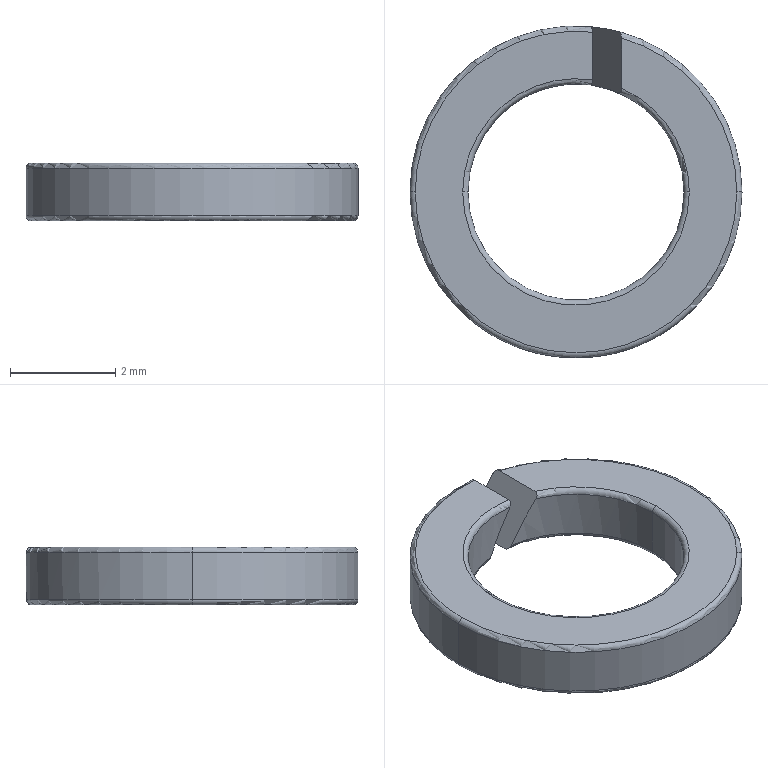Part | STEP file | 弹垫-4^EDA50-R04 (D60N) | 1 solid | 22 faces | box 6.3 x 6.3 x 1.1 mm | volume 18.959 mm3 | torus 12 | cylinder 6 | plane 4 | commonest cylinder face diameters 4.1 x3 6.3 x3